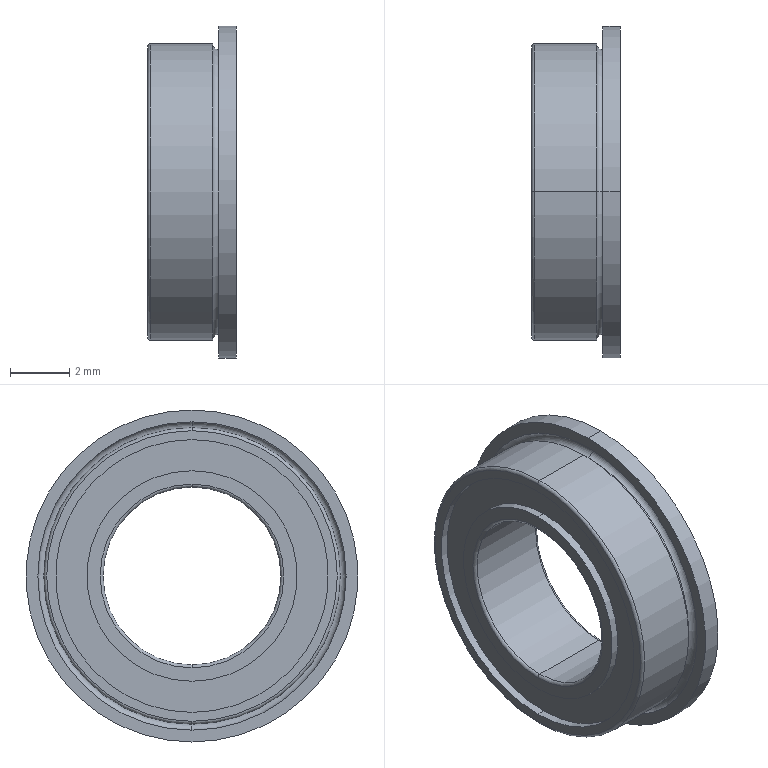Part | NX | features BREP 1 | 1 solid | 31 faces | box 3 x 11.2 x 11.2 mm | volume 145.175 mm3 | cylinder 14 | torus 10 | plane 7 | commonest cylinder face diameters 7.1 x4 9.2 x4 6 x2 10 x2 11.2 x2
STEP:
#1=CARTESIAN_POINT('',(0.,0.,4.8));
#2=VERTEX_POINT('',#1);
#3=CARTESIAN_POINT('',(-0.2,0.,5.));
#4=VERTEX_POINT('',#3);
#5=CARTESIAN_POINT('',(0.,0.,5.));
#6=DIRECTION('',(0.,-1.,0.));
#7=DIRECTION('',(0.,0.,-1.));
#8=AXIS2_PLACEMENT_3D('',#5,#6,#7);
#9=CIRCLE('',#8,0.2);
#10=EDGE_CURVE('',#2,#4,#9,.F.);
#11=ORIENTED_EDGE('',*,*,#10,.F.);
#12=CARTESIAN_POINT('',(0.,0.,-4.8));
#13=VERTEX_POINT('',#12);
#14=CARTESIAN_POINT('',(0.,0.,0.));
#15=DIRECTION('',(-1.,0.,0.));
#16=DIRECTION('',(0.,0.,1.));
#17=AXIS2_PLACEMENT_3D('',#14,#15,#16);
#18=CIRCLE('',#17,4.8);
#19=EDGE_CURVE('',#2,#13,#18,.T.);
#20=ORIENTED_EDGE('',*,*,#19,.T.);
#21=CARTESIAN_POINT('',(-0.2,0.,-5.));
#22=VERTEX_POINT('',#21);
#23=CARTESIAN_POINT('',(0.,0.,-5.));
#24=DIRECTION('',(0.,1.,0.));
#25=DIRECTION('',(0.,0.,1.));
#26=AXIS2_PLACEMENT_3D('',#23,#24,#25);
#27=CIRCLE('',#26,0.2);
#28=EDGE_CURVE('',#13,#22,#27,.F.);
#29=ORIENTED_EDGE('',*,*,#28,.T.);
#30=CARTESIAN_POINT('',(-0.2,0.,0.));
#31=DIRECTION('',(-1.,0.,0.));
#32=DIRECTION('',(0.,0.,1.));
#33=AXIS2_PLACEMENT_3D('',#30,#31,#32);
#34=CIRCLE('',#33,5.);
#35=EDGE_CURVE('',#4,#22,#34,.T.);
#36=ORIENTED_EDGE('',*,*,#35,.F.);
#37=EDGE_LOOP('',(#11,#20,#29,#36));
#38=FACE_BOUND('',#37,.T.);
#39=CARTESIAN_POINT('',(0.,0.,0.));
#40=DIRECTION('',(-1.,0.,0.));
#41=DIRECTION('',(0.,0.,-1.));
#42=AXIS2_PLACEMENT_3D('',#39,#40,#41);
#43=TOROIDAL_SURFACE('',#42,5.,0.2);
#44=ADVANCED_FACE('',(#38),#43,.F.);
#45=ORIENTED_EDGE('',*,*,#28,.F.);
#46=CARTESIAN_POINT('',(0.,0.,0.));
#47=DIRECTION('',(-1.,0.,0.));
#48=DIRECTION('',(0.,0.,1.));
#49=AXIS2_PLACEMENT_3D('',#46,#47,#48);
#50=CIRCLE('',#49,4.8);
#51=EDGE_CURVE('',#13,#2,#50,.T.);
#52=ORIENTED_EDGE('',*,*,#51,.T.);
#53=ORIENTED_EDGE('',*,*,#10,.T.);
#54=CARTESIAN_POINT('',(-0.2,0.,0.));
#55=DIRECTION('',(-1.,0.,0.));
#56=DIRECTION('',(0.,0.,1.));
#57=AXIS2_PLACEMENT_3D('',#54,#55,#56);
#58=CIRCLE('',#57,5.);
#59=EDGE_CURVE('',#22,#4,#58,.T.);
#60=ORIENTED_EDGE('',*,*,#59,.F.);
#61=EDGE_LOOP('',(#45,#52,#53,#60));
#62=FACE_BOUND('',#61,.T.);
#63=CARTESIAN_POINT('',(0.,0.,0.));
#64=DIRECTION('',(-1.,0.,0.));
#65=DIRECTION('',(0.,0.,-1.));
#66=AXIS2_PLACEMENT_3D('',#63,#64,#65);
#67=TOROIDAL_SURFACE('',#66,5.,0.2);
#68=ADVANCED_FACE('',(#62),#67,.F.);
#69=CARTESIAN_POINT('',(0.6,0.,-4.6));
#70=VERTEX_POINT('',#69);
#71=CARTESIAN_POINT('',(0.6,0.,4.6));
#72=VERTEX_POINT('',#71);
#73=CARTESIAN_POINT('',(0.6,0.,0.));
#74=DIRECTION('',(-1.,0.,0.));
#75=DIRECTION('',(0.,0.,1.));
#76=AXIS2_PLACEMENT_3D('',#73,#74,#75);
#77=CIRCLE('',#76,4.6);
#78=EDGE_CURVE('',#70,#72,#77,.T.);
#79=ORIENTED_EDGE('',*,*,#78,.F.);
#80=CARTESIAN_POINT('',(0.33,0.,-4.6));
#81=VERTEX_POINT('',#80);
#82=CARTESIAN_POINT('',(-1.815,0.,-4.6));
#83=DIRECTION('',(-1.,0.,0.));
#84=VECTOR('',#83,1000.);
#85=LINE('',#82,#84);
#86=EDGE_CURVE('',#70,#81,#85,.T.);
#87=ORIENTED_EDGE('',*,*,#86,.T.);
#88=CARTESIAN_POINT('',(0.33,0.,4.6));
#89=VERTEX_POINT('',#88);
#90=CARTESIAN_POINT('',(0.33,0.,0.));
#91=DIRECTION('',(-1.,0.,0.));
#92=DIRECTION('',(0.,0.,1.));
#93=AXIS2_PLACEMENT_3D('',#90,#91,#92);
#94=CIRCLE('',#93,4.6);
#95=EDGE_CURVE('',#81,#89,#94,.T.);
#96=ORIENTED_EDGE('',*,*,#95,.T.);
#97=CARTESIAN_POINT('',(-1.815,0.,4.6));
#98=DIRECTION('',(-1.,0.,0.));
#99=VECTOR('',#98,1000.);
#100=LINE('',#97,#99);
#101=EDGE_CURVE('',#72,#89,#100,.T.);
#102=ORIENTED_EDGE('',*,*,#101,.F.);
#103=EDGE_LOOP('',(#79,#87,#96,#102));
#104=FACE_BOUND('',#103,.T.);
#105=CARTESIAN_POINT('',(-1.815,0.,0.));
#106=DIRECTION('',(-1.,0.,0.));
#107=DIRECTION('',(0.,0.,-1.));
#108=AXIS2_PLACEMENT_3D('',#105,#106,#107);
#109=CYLINDRICAL_SURFACE('',#108,4.6);
#110=ADVANCED_FACE('',(#104),#109,.F.);
#111=CARTESIAN_POINT('',(0.6,0.,3.55));
#112=VERTEX_POINT('',#111);
#113=CARTESIAN_POINT('',(0.6,0.,-3.55));
#114=VERTEX_POINT('',#113);
#115=CARTESIAN_POINT('',(0.6,0.,0.));
#116=DIRECTION('',(-1.,0.,0.));
#117=DIRECTION('',(0.,0.,1.));
#118=AXIS2_PLACEMENT_3D('',#115,#116,#117);
#119=CIRCLE('',#118,3.55);
#120=EDGE_CURVE('',#112,#114,#119,.T.);
#121=ORIENTED_EDGE('',*,*,#120,.T.);
#122=CARTESIAN_POINT('',(0.33,0.,-3.55));
#123=VERTEX_POINT('',#122);
#124=CARTESIAN_POINT('',(-1.815,0.,-3.55));
#125=DIRECTION('',(-1.,0.,0.));
#126=VECTOR('',#125,1000.);
#127=LINE('',#124,#126);
#128=EDGE_CURVE('',#114,#123,#127,.T.);
#129=ORIENTED_EDGE('',*,*,#128,.T.);
#130=CARTESIAN_POINT('',(0.33,0.,3.55));
#131=VERTEX_POINT('',#130);
#132=CARTESIAN_POINT('',(0.33,0.,0.));
#133=DIRECTION('',(-1.,0.,0.));
#134=DIRECTION('',(0.,0.,1.));
#135=AXIS2_PLACEMENT_3D('',#132,#133,#134);
#136=CIRCLE('',#135,3.55);
#137=EDGE_CURVE('',#131,#123,#136,.T.);
#138=ORIENTED_EDGE('',*,*,#137,.F.);
#139=CARTESIAN_POINT('',(-1.815,0.,3.55));
#140=DIRECTION('',(-1.,0.,0.));
#141=VECTOR('',#140,1000.);
#142=LINE('',#139,#141);
#143=EDGE_CURVE('',#112,#131,#142,.T.);
#144=ORIENTED_EDGE('',*,*,#143,.F.);
#145=EDGE_LOOP('',(#121,#129,#138,#144));
#146=FACE_BOUND('',#145,.T.);
#147=CARTESIAN_POINT('',(-1.815,0.,0.));
#148=DIRECTION('',(-1.,0.,0.));
#149=DIRECTION('',(0.,0.,-1.));
#150=AXIS2_PLACEMENT_3D('',#147,#148,#149);
#151=CYLINDRICAL_SURFACE('',#150,3.55);
#152=ADVANCED_FACE('',(#146),#151,.T.);
#153=CARTESIAN_POINT('',(0.5,0.,3.));
#154=VERTEX_POINT('',#153);
#155=CARTESIAN_POINT('',(0.5,0.,-3.));
#156=VERTEX_POINT('',#155);
#157=CARTESIAN_POINT('',(0.5,0.,0.));
#158=DIRECTION('',(-1.,0.,0.));
#159=DIRECTION('',(0.,0.,1.));
#160=AXIS2_PLACEMENT_3D('',#157,#158,#159);
#161=CIRCLE('',#160,3.);
#162=EDGE_CURVE('',#154,#156,#161,.T.);
#163=ORIENTED_EDGE('',*,*,#162,.T.);
#164=CARTESIAN_POINT('',(0.6,0.,-3.1));
#165=VERTEX_POINT('',#164);
#166=CARTESIAN_POINT('',(0.5,0.,-3.1));
#167=DIRECTION('',(0.,1.,0.));
#168=DIRECTION('',(0.,0.,1.));
#169=AXIS2_PLACEMENT_3D('',#166,#167,#168);
#170=CIRCLE('',#169,0.1);
#171=EDGE_CURVE('',#156,#165,#170,.T.);
#172=ORIENTED_EDGE('',*,*,#171,.T.);
#173=CARTESIAN_POINT('',(0.6,0.,3.1));
#174=VERTEX_POINT('',#173);
#175=CARTESIAN_POINT('',(0.6,0.,0.));
#176=DIRECTION('',(-1.,0.,0.));
#177=DIRECTION('',(0.,0.,1.));
#178=AXIS2_PLACEMENT_3D('',#175,#176,#177);
#179=CIRCLE('',#178,3.1);
#180=EDGE_CURVE('',#174,#165,#179,.T.);
#181=ORIENTED_EDGE('',*,*,#180,.F.);
#182=CARTESIAN_POINT('',(0.5,0.,3.1));
#183=DIRECTION('',(0.,-1.,0.));
#184=DIRECTION('',(0.,0.,-1.));
#185=AXIS2_PLACEMENT_3D('',#182,#183,#184);
#186=CIRCLE('',#185,0.1);
#187=EDGE_CURVE('',#154,#174,#186,.T.);
#188=ORIENTED_EDGE('',*,*,#187,.F.);
#189=EDGE_LOOP('',(#163,#172,#181,#188));
#190=FACE_BOUND('',#189,.T.);
#191=CARTESIAN_POINT('',(0.5,0.,0.));
#192=DIRECTION('',(-1.,0.,0.));
#193=DIRECTION('',(0.,0.,-1.));
#194=AXIS2_PLACEMENT_3D('',#191,#192,#193);
#195=TOROIDAL_SURFACE('',#194,3.1,0.1);
#196=ADVANCED_FACE('',(#190),#195,.T.);
#197=CARTESIAN_POINT('',(0.5,0.,0.));
#198=DIRECTION('',(-1.,0.,0.));
#199=DIRECTION('',(0.,0.,1.));
#200=AXIS2_PLACEMENT_3D('',#197,#198,#199);
#201=CIRCLE('',#200,3.);
#202=EDGE_CURVE('',#156,#154,#201,.T.);
#203=ORIENTED_EDGE('',*,*,#202,.F.);
#204=CARTESIAN_POINT('',(-2.3,0.,-3.));
#205=VERTEX_POINT('',#204);
#206=CARTESIAN_POINT('',(-1.815,0.,-3.));
#207=DIRECTION('',(-1.,0.,0.));
#208=VECTOR('',#207,1000.);
#209=LINE('',#206,#208);
#210=EDGE_CURVE('',#156,#205,#209,.T.);
#211=ORIENTED_EDGE('',*,*,#210,.T.);
#212=CARTESIAN_POINT('',(-2.3,0.,3.));
#213=VERTEX_POINT('',#212);
#214=CARTESIAN_POINT('',(-2.3,0.,0.));
#215=DIRECTION('',(-1.,0.,0.));
#216=DIRECTION('',(0.,0.,1.));
#217=AXIS2_PLACEMENT_3D('',#214,#215,#216);
#218=CIRCLE('',#217,3.);
#219=EDGE_CURVE('',#205,#213,#218,.T.);
#220=ORIENTED_EDGE('',*,*,#219,.T.);
#221=CARTESIAN_POINT('',(-1.815,0.,3.));
#222=DIRECTION('',(-1.,0.,0.));
#223=VECTOR('',#222,1000.);
#224=LINE('',#221,#223);
#225=EDGE_CURVE('',#154,#213,#224,.T.);
#226=ORIENTED_EDGE('',*,*,#225,.F.);
#227=EDGE_LOOP('',(#203,#211,#220,#226));
#228=FACE_BOUND('',#227,.T.);
#229=CARTESIAN_POINT('',(-1.815,0.,0.));
#230=DIRECTION('',(-1.,0.,0.));
#231=DIRECTION('',(0.,0.,-1.));
#232=AXIS2_PLACEMENT_3D('',#229,#230,#231);
#233=CYLINDRICAL_SURFACE('',#232,3.);
#234=ADVANCED_FACE('',(#228),#233,.F.);
#235=CARTESIAN_POINT('',(-2.4,0.,3.1));
#236=VERTEX_POINT('',#235);
#237=CARTESIAN_POINT('',(-2.4,0.,-3.1));
#238=VERTEX_POINT('',#237);
#239=CARTESIAN_POINT('',(-2.4,0.,0.));
#240=DIRECTION('',(-1.,0.,0.));
#241=DIRECTION('',(0.,0.,1.));
#242=AXIS2_PLACEMENT_3D('',#239,#240,#241);
#243=CIRCLE('',#242,3.1);
#244=EDGE_CURVE('',#236,#238,#243,.T.);
#245=ORIENTED_EDGE('',*,*,#244,.T.);
#246=CARTESIAN_POINT('',(-2.3,0.,-3.1));
#247=DIRECTION('',(0.,1.,0.));
#248=DIRECTION('',(0.,0.,1.));
#249=AXIS2_PLACEMENT_3D('',#246,#247,#248);
#250=CIRCLE('',#249,0.1);
#251=EDGE_CURVE('',#238,#205,#250,.T.);
#252=ORIENTED_EDGE('',*,*,#251,.T.);
#253=CARTESIAN_POINT('',(-2.3,0.,0.));
#254=DIRECTION('',(-1.,0.,0.));
#255=DIRECTION('',(0.,0.,1.));
#256=AXIS2_PLACEMENT_3D('',#253,#254,#255);
#257=CIRCLE('',#256,3.);
#258=EDGE_CURVE('',#213,#205,#257,.T.);
#259=ORIENTED_EDGE('',*,*,#258,.F.);
#260=CARTESIAN_POINT('',(-2.3,0.,3.1));
#261=DIRECTION('',(0.,-1.,0.));
#262=DIRECTION('',(0.,0.,-1.));
#263=AXIS2_PLACEMENT_3D('',#260,#261,#262);
#264=CIRCLE('',#263,0.1);
#265=EDGE_CURVE('',#236,#213,#264,.T.);
#266=ORIENTED_EDGE('',*,*,#265,.F.);
#267=EDGE_LOOP('',(#245,#252,#259,#266));
#268=FACE_BOUND('',#267,.T.);
#269=CARTESIAN_POINT('',(-2.3,0.,0.));
#270=DIRECTION('',(-1.,0.,0.));
#271=DIRECTION('',(0.,0.,-1.));
#272=AXIS2_PLACEMENT_3D('',#269,#270,#271);
#273=TOROIDAL_SURFACE('',#272,3.1,0.1);
#274=ADVANCED_FACE('',(#268),#273,.T.);
#275=CARTESIAN_POINT('',(-2.13,0.,3.55));
#276=VERTEX_POINT('',#275);
#277=CARTESIAN_POINT('',(-2.13,0.,-3.55));
#278=VERTEX_POINT('',#277);
#279=CARTESIAN_POINT('',(-2.13,0.,0.));
#280=DIRECTION('',(-1.,0.,0.));
#281=DIRECTION('',(0.,0.,1.));
#282=AXIS2_PLACEMENT_3D('',#279,#280,#281);
#283=CIRCLE('',#282,3.55);
#284=EDGE_CURVE('',#276,#278,#283,.T.);
#285=ORIENTED_EDGE('',*,*,#284,.T.);
#286=CARTESIAN_POINT('',(-2.4,0.,-3.55));
#287=VERTEX_POINT('',#286);
#288=CARTESIAN_POINT('',(-1.815,0.,-3.55));
#289=DIRECTION('',(-1.,0.,0.));
#290=VECTOR('',#289,1000.);
#291=LINE('',#288,#290);
#292=EDGE_CURVE('',#278,#287,#291,.T.);
#293=ORIENTED_EDGE('',*,*,#292,.T.);
#294=CARTESIAN_POINT('',(-2.4,0.,3.55));
#295=VERTEX_POINT('',#294);
#296=CARTESIAN_POINT('',(-2.4,0.,0.));
#297=DIRECTION('',(-1.,0.,0.));
#298=DIRECTION('',(0.,0.,1.));
#299=AXIS2_PLACEMENT_3D('',#296,#297,#298);
#300=CIRCLE('',#299,3.55);
#301=EDGE_CURVE('',#295,#287,#300,.T.);
#302=ORIENTED_EDGE('',*,*,#301,.F.);
#303=CARTESIAN_POINT('',(-1.815,0.,3.55));
#304=DIRECTION('',(-1.,0.,0.));
#305=VECTOR('',#304,1000.);
#306=LINE('',#303,#305);
#307=EDGE_CURVE('',#276,#295,#306,.T.);
#308=ORIENTED_EDGE('',*,*,#307,.F.);
#309=EDGE_LOOP('',(#285,#293,#302,#308));
#310=FACE_BOUND('',#309,.T.);
#311=CARTESIAN_POINT('',(-1.815,0.,0.));
#312=DIRECTION('',(-1.,0.,0.));
#313=DIRECTION('',(0.,0.,-1.));
#314=AXIS2_PLACEMENT_3D('',#311,#312,#313);
#315=CYLINDRICAL_SURFACE('',#314,3.55);
#316=ADVANCED_FACE('',(#310),#315,.T.);
#317=CARTESIAN_POINT('',(-2.13,0.,-4.6));
#318=VERTEX_POINT('',#317);
#319=CARTESIAN_POINT('',(-2.13,0.,4.6));
#320=VERTEX_POINT('',#319);
#321=CARTESIAN_POINT('',(-2.13,0.,0.));
#322=DIRECTION('',(-1.,0.,0.));
#323=DIRECTION('',(0.,0.,1.));
#324=AXIS2_PLACEMENT_3D('',#321,#322,#323);
#325=CIRCLE('',#324,4.6);
#326=EDGE_CURVE('',#318,#320,#325,.T.);
#327=ORIENTED_EDGE('',*,*,#326,.F.);
#328=CARTESIAN_POINT('',(-2.4,0.,-4.6));
#329=VERTEX_POINT('',#328);
#330=CARTESIAN_POINT('',(-1.815,0.,-4.6));
#331=DIRECTION('',(-1.,0.,0.));
#332=VECTOR('',#331,1000.);
#333=LINE('',#330,#332);
#334=EDGE_CURVE('',#318,#329,#333,.T.);
#335=ORIENTED_EDGE('',*,*,#334,.T.);
#336=CARTESIAN_POINT('',(-2.4,0.,4.6));
#337=VERTEX_POINT('',#336);
#338=CARTESIAN_POINT('',(-2.4,0.,0.));
#339=DIRECTION('',(-1.,0.,0.));
#340=DIRECTION('',(0.,0.,1.));
#341=AXIS2_PLACEMENT_3D('',#338,#339,#340);
#342=CIRCLE('',#341,4.6);
#343=EDGE_CURVE('',#329,#337,#342,.T.);
#344=ORIENTED_EDGE('',*,*,#343,.T.);
#345=CARTESIAN_POINT('',(-1.815,0.,4.6));
#346=DIRECTION('',(-1.,0.,0.));
#347=VECTOR('',#346,1000.);
#348=LINE('',#345,#347);
#349=EDGE_CURVE('',#320,#337,#348,.T.);
#350=ORIENTED_EDGE('',*,*,#349,.F.);
#351=EDGE_LOOP('',(#327,#335,#344,#350));
#352=FACE_BOUND('',#351,.T.);
#353=CARTESIAN_POINT('',(-1.815,0.,0.));
#354=DIRECTION('',(-1.,0.,0.));
#355=DIRECTION('',(0.,0.,-1.));
#356=AXIS2_PLACEMENT_3D('',#353,#354,#355);
#357=CYLINDRICAL_SURFACE('',#356,4.6);
#358=ADVANCED_FACE('',(#352),#357,.F.);
#359=CARTESIAN_POINT('',(-2.3,0.,5.));
#360=VERTEX_POINT('',#359);
#361=CARTESIAN_POINT('',(-2.3,0.,-5.));
#362=VERTEX_POINT('',#361);
#363=CARTESIAN_POINT('',(-2.3,0.,0.));
#364=DIRECTION('',(-1.,0.,0.));
#365=DIRECTION('',(0.,0.,1.));
#366=AXIS2_PLACEMENT_3D('',#363,#364,#365);
#367=CIRCLE('',#366,5.);
#368=EDGE_CURVE('',#360,#362,#367,.T.);
#369=ORIENTED_EDGE('',*,*,#368,.T.);
#370=CARTESIAN_POINT('',(-2.4,0.,-4.9));
#371=VERTEX_POINT('',#370);
#372=CARTESIAN_POINT('',(-2.3,0.,-4.9));
#373=DIRECTION('',(0.,1.,0.));
#374=DIRECTION('',(0.,0.,1.));
#375=AXIS2_PLACEMENT_3D('',#372,#373,#374);
#376=CIRCLE('',#375,0.1);
#377=EDGE_CURVE('',#362,#371,#376,.T.);
#378=ORIENTED_EDGE('',*,*,#377,.T.);
#379=CARTESIAN_POINT('',(-2.4,0.,4.9));
#380=VERTEX_POINT('',#379);
#381=CARTESIAN_POINT('',(-2.4,0.,0.));
#382=DIRECTION('',(-1.,0.,0.));
#383=DIRECTION('',(0.,0.,1.));
#384=AXIS2_PLACEMENT_3D('',#381,#382,#383);
#385=CIRCLE('',#384,4.9);
#386=EDGE_CURVE('',#380,#371,#385,.T.);
#387=ORIENTED_EDGE('',*,*,#386,.F.);
#388=CARTESIAN_POINT('',(-2.3,0.,4.9));
#389=DIRECTION('',(0.,-1.,0.));
#390=DIRECTION('',(0.,0.,-1.));
#391=AXIS2_PLACEMENT_3D('',#388,#389,#390);
#392=CIRCLE('',#391,0.1);
#393=EDGE_CURVE('',#360,#380,#392,.T.);
#394=ORIENTED_EDGE('',*,*,#393,.F.);
#395=EDGE_LOOP('',(#369,#378,#387,#394));
#396=FACE_BOUND('',#395,.T.);
#397=CARTESIAN_POINT('',(-2.3,0.,0.));
#398=DIRECTION('',(-1.,0.,0.));
#399=DIRECTION('',(0.,0.,-1.));
#400=AXIS2_PLACEMENT_3D('',#397,#398,#399);
#401=TOROIDAL_SURFACE('',#400,4.9,0.1);
#402=ADVANCED_FACE('',(#396),#401,.T.);
#403=ORIENTED_EDGE('',*,*,#35,.T.);
#404=CARTESIAN_POINT('',(-1.815,0.,-5.));
#405=DIRECTION('',(-1.,0.,0.));
#406=VECTOR('',#405,1000.);
#407=LINE('',#404,#406);
#408=EDGE_CURVE('',#22,#362,#407,.T.);
#409=ORIENTED_EDGE('',*,*,#408,.T.);
#410=ORIENTED_EDGE('',*,*,#368,.F.);
#411=CARTESIAN_POINT('',(-1.815,0.,5.));
#412=DIRECTION('',(-1.,0.,0.));
#413=VECTOR('',#412,1000.);
#414=LINE('',#411,#413);
#415=EDGE_CURVE('',#4,#360,#414,.T.);
#416=ORIENTED_EDGE('',*,*,#415,.F.);
#417=EDGE_LOOP('',(#403,#409,#410,#416));
#418=FACE_BOUND('',#417,.T.);
#419=CARTESIAN_POINT('',(-1.815,0.,0.));
#420=DIRECTION('',(-1.,0.,0.));
#421=DIRECTION('',(0.,0.,-1.));
#422=AXIS2_PLACEMENT_3D('',#419,#420,#421);
#423=CYLINDRICAL_SURFACE('',#422,5.);
#424=ADVANCED_FACE('',(#418),#423,.T.);
#425=ORIENTED_EDGE('',*,*,#51,.F.);
#426=CARTESIAN_POINT('',(0.,0.,-5.2));
#427=VERTEX_POINT('',#426);
#428=CARTESIAN_POINT('',(0.,0.,-5.));
#429=DIRECTION('',(0.,1.,0.));
#430=DIRECTION('',(0.,0.,1.));
#431=AXIS2_PLACEMENT_3D('',#428,#429,#430);
#432=CIRCLE('',#431,0.2);
#433=EDGE_CURVE('',#13,#427,#432,.T.);
#434=ORIENTED_EDGE('',*,*,#433,.T.);
#435=CARTESIAN_POINT('',(0.,0.,5.2));
#436=VERTEX_POINT('',#435);
#437=CARTESIAN_POINT('',(0.,0.,0.));
#438=DIRECTION('',(-1.,0.,0.));
#439=DIRECTION('',(0.,0.,1.));
#440=AXIS2_PLACEMENT_3D('',#437,#438,#439);
#441=CIRCLE('',#440,5.2);
#442=EDGE_CURVE('',#427,#436,#441,.T.);
#443=ORIENTED_EDGE('',*,*,#442,.T.);
#444=CARTESIAN_POINT('',(0.,0.,5.));
#445=DIRECTION('',(0.,-1.,0.));
#446=DIRECTION('',(0.,0.,-1.));
#447=AXIS2_PLACEMENT_3D('',#444,#445,#446);
#448=CIRCLE('',#447,0.2);
#449=EDGE_CURVE('',#2,#436,#448,.T.);
#450=ORIENTED_EDGE('',*,*,#449,.F.);
#451=EDGE_LOOP('',(#425,#434,#443,#450));
#452=FACE_BOUND('',#451,.T.);
#453=CARTESIAN_POINT('',(0.,0.,0.));
#454=DIRECTION('',(-1.,0.,0.));
#455=DIRECTION('',(0.,0.,-1.));
#456=AXIS2_PLACEMENT_3D('',#453,#454,#455);
#457=TOROIDAL_SURFACE('',#456,5.,0.2);
#458=ADVANCED_FACE('',(#452),#457,.F.);
#459=CARTESIAN_POINT('',(0.6,0.,5.6));
#460=VERTEX_POINT('',#459);
#461=CARTESIAN_POINT('',(0.6,0.,-5.6));
#462=VERTEX_POINT('',#461);
#463=CARTESIAN_POINT('',(0.6,0.,0.));
#464=DIRECTION('',(-1.,0.,0.));
#465=DIRECTION('',(0.,0.,1.));
#466=AXIS2_PLACEMENT_3D('',#463,#464,#465);
#467=CIRCLE('',#466,5.6);
#468=EDGE_CURVE('',#460,#462,#467,.T.);
#469=ORIENTED_EDGE('',*,*,#468,.T.);
#470=CARTESIAN_POINT('',(0.,0.,-5.6));
#471=VERTEX_POINT('',#470);
#472=CARTESIAN_POINT('',(-1.815,0.,-5.6));
#473=DIRECTION('',(-1.,0.,0.));
#474=VECTOR('',#473,1000.);
#475=LINE('',#472,#474);
#476=EDGE_CURVE('',#462,#471,#475,.T.);
#477=ORIENTED_EDGE('',*,*,#476,.T.);
#478=CARTESIAN_POINT('',(0.,0.,5.6));
#479=VERTEX_POINT('',#478);
#480=CARTESIAN_POINT('',(0.,0.,0.));
#481=DIRECTION('',(-1.,0.,0.));
#482=DIRECTION('',(0.,0.,1.));
#483=AXIS2_PLACEMENT_3D('',#480,#481,#482);
#484=CIRCLE('',#483,5.6);
#485=EDGE_CURVE('',#479,#471,#484,.T.);
#486=ORIENTED_EDGE('',*,*,#485,.F.);
#487=CARTESIAN_POINT('',(-1.815,0.,5.6));
#488=DIRECTION('',(-1.,0.,0.));
#489=VECTOR('',#488,1000.);
#490=LINE('',#487,#489);
#491=EDGE_CURVE('',#460,#479,#490,.T.);
#492=ORIENTED_EDGE('',*,*,#491,.F.);
#493=EDGE_LOOP('',(#469,#477,#486,#492));
#494=FACE_BOUND('',#493,.T.);
#495=CARTESIAN_POINT('',(-1.815,0.,0.));
#496=DIRECTION('',(-1.,0.,0.));
#497=DIRECTION('',(0.,0.,-1.));
#498=AXIS2_PLACEMENT_3D('',#495,#496,#497);
#499=CYLINDRICAL_SURFACE('',#498,5.6);
#500=ADVANCED_FACE('',(#494),#499,.T.);
#501=ORIENTED_EDGE('',*,*,#476,.F.);
#502=CARTESIAN_POINT('',(0.6,0.,0.));
#503=DIRECTION('',(-1.,0.,0.));
#504=DIRECTION('',(0.,0.,1.));
#505=AXIS2_PLACEMENT_3D('',#502,#503,#504);
#506=CIRCLE('',#505,5.6);
#507=EDGE_CURVE('',#462,#460,#506,.T.);
#508=ORIENTED_EDGE('',*,*,#507,.T.);
#509=ORIENTED_EDGE('',*,*,#491,.T.);
#510=CARTESIAN_POINT('',(0.,0.,0.));
#511=DIRECTION('',(-1.,0.,0.));
#512=DIRECTION('',(0.,0.,1.));
#513=AXIS2_PLACEMENT_3D('',#510,#511,#512);
#514=CIRCLE('',#513,5.6);
#515=EDGE_CURVE('',#471,#479,#514,.T.);
#516=ORIENTED_EDGE('',*,*,#515,.F.);
#517=EDGE_LOOP('',(#501,#508,#509,#516));
#518=FACE_BOUND('',#517,.T.);
#519=CARTESIAN_POINT('',(-1.815,0.,0.));
#520=DIRECTION('',(-1.,0.,0.));
#521=DIRECTION('',(0.,0.,-1.));
#522=AXIS2_PLACEMENT_3D('',#519,#520,#521);
#523=CYLINDRICAL_SURFACE('',#522,5.6);
#524=ADVANCED_FACE('',(#518),#523,.T.);
#525=ORIENTED_EDGE('',*,*,#485,.T.);
#526=ORIENTED_EDGE('',*,*,#515,.T.);
#527=EDGE_LOOP('',(#525,#526));
#528=FACE_BOUND('',#527,.T.);
#529=CARTESIAN_POINT('',(0.,0.,0.));
#530=DIRECTION('',(-1.,0.,0.));
#531=DIRECTION('',(0.,0.,1.));
#532=AXIS2_PLACEMENT_3D('',#529,#530,#531);
#533=CIRCLE('',#532,5.2);
#534=EDGE_CURVE('',#436,#427,#533,.T.);
#535=ORIENTED_EDGE('',*,*,#534,.F.);
#536=ORIENTED_EDGE('',*,*,#442,.F.);
#537=EDGE_LOOP('',(#535,#536));
#538=FACE_BOUND('',#537,.T.);
#539=CARTESIAN_POINT('',(0.,5.2,0.));
#540=DIRECTION('',(1.,0.,0.));
#541=DIRECTION('',(0.,-1.,0.));
#542=AXIS2_PLACEMENT_3D('',#539,#540,#541);
#543=PLANE('',#542);
#544=ADVANCED_FACE('',(#528,#538),#543,.F.);
#545=ORIENTED_EDGE('',*,*,#19,.F.);
#546=ORIENTED_EDGE('',*,*,#449,.T.);
#547=ORIENTED_EDGE('',*,*,#534,.T.);
#548=ORIENTED_EDGE('',*,*,#433,.F.);
#549=EDGE_LOOP('',(#545,#546,#547,#548));
#550=FACE_BOUND('',#549,.T.);
#551=CARTESIAN_POINT('',(0.,0.,0.));
#552=DIRECTION('',(-1.,0.,0.));
#553=DIRECTION('',(0.,0.,-1.));
#554=AXIS2_PLACEMENT_3D('',#551,#552,#553);
#555=TOROIDAL_SURFACE('',#554,5.,0.2);
#556=ADVANCED_FACE('',(#550),#555,.F.);
#557=ORIENTED_EDGE('',*,*,#408,.F.);
#558=ORIENTED_EDGE('',*,*,#59,.T.);
#559=ORIENTED_EDGE('',*,*,#415,.T.);
#560=CARTESIAN_POINT('',(-2.3,0.,0.));
#561=DIRECTION('',(-1.,0.,0.));
#562=DIRECTION('',(0.,0.,1.));
#563=AXIS2_PLACEMENT_3D('',#560,#561,#562);
#564=CIRCLE('',#563,5.);
#565=EDGE_CURVE('',#362,#360,#564,.T.);
#566=ORIENTED_EDGE('',*,*,#565,.F.);
#567=EDGE_LOOP('',(#557,#558,#559,#566));
#568=FACE_BOUND('',#567,.T.);
#569=CARTESIAN_POINT('',(-1.815,0.,0.));
#570=DIRECTION('',(-1.,0.,0.));
#571=DIRECTION('',(0.,0.,-1.));
#572=AXIS2_PLACEMENT_3D('',#569,#570,#571);
#573=CYLINDRICAL_SURFACE('',#572,5.);
#574=ADVANCED_FACE('',(#568),#573,.T.);
#575=ORIENTED_EDGE('',*,*,#377,.F.);
#576=ORIENTED_EDGE('',*,*,#565,.T.);
#577=ORIENTED_EDGE('',*,*,#393,.T.);
#578=CARTESIAN_POINT('',(-2.4,0.,0.));
#579=DIRECTION('',(-1.,0.,0.));
#580=DIRECTION('',(0.,0.,1.));
#581=AXIS2_PLACEMENT_3D('',#578,#579,#580);
#582=CIRCLE('',#581,4.9);
#583=EDGE_CURVE('',#371,#380,#582,.T.);
#584=ORIENTED_EDGE('',*,*,#583,.F.);
#585=EDGE_LOOP('',(#575,#576,#577,#584));
#586=FACE_BOUND('',#585,.T.);
#587=CARTESIAN_POINT('',(-2.3,0.,0.));
#588=DIRECTION('',(-1.,0.,0.));
#589=DIRECTION('',(0.,0.,-1.));
#590=AXIS2_PLACEMENT_3D('',#587,#588,#589);
#591=TOROIDAL_SURFACE('',#590,4.9,0.1);
#592=ADVANCED_FACE('',(#586),#591,.T.);
#593=ORIENTED_EDGE('',*,*,#386,.T.);
#594=ORIENTED_EDGE('',*,*,#583,.T.);
#595=EDGE_LOOP('',(#593,#594));
#596=FACE_BOUND('',#595,.T.);
#597=CARTESIAN_POINT('',(-2.4,0.,0.));
#598=DIRECTION('',(-1.,0.,0.));
#599=DIRECTION('',(0.,0.,1.));
#600=AXIS2_PLACEMENT_3D('',#597,#598,#599);
#601=CIRCLE('',#600,4.6);
#602=EDGE_CURVE('',#337,#329,#601,.T.);
#603=ORIENTED_EDGE('',*,*,#602,.F.);
#604=ORIENTED_EDGE('',*,*,#343,.F.);
#605=EDGE_LOOP('',(#603,#604));
#606=FACE_BOUND('',#605,.T.);
#607=CARTESIAN_POINT('',(-2.4,4.6,0.));
#608=DIRECTION('',(1.,0.,0.));
#609=DIRECTION('',(0.,-1.,0.));
#610=AXIS2_PLACEMENT_3D('',#607,#608,#609);
#611=PLANE('',#610);
#612=ADVANCED_FACE('',(#596,#606),#611,.F.);
#613=ORIENTED_EDGE('',*,*,#334,.F.);
#614=CARTESIAN_POINT('',(-2.13,0.,0.));
#615=DIRECTION('',(-1.,0.,0.));
#616=DIRECTION('',(0.,0.,1.));
#617=AXIS2_PLACEMENT_3D('',#614,#615,#616);
#618=CIRCLE('',#617,4.6);
#619=EDGE_CURVE('',#320,#318,#618,.T.);
#620=ORIENTED_EDGE('',*,*,#619,.F.);
#621=ORIENTED_EDGE('',*,*,#349,.T.);
#622=ORIENTED_EDGE('',*,*,#602,.T.);
#623=EDGE_LOOP('',(#613,#620,#621,#622));
#624=FACE_BOUND('',#623,.T.);
#625=CARTESIAN_POINT('',(-1.815,0.,0.));
#626=DIRECTION('',(-1.,0.,0.));
#627=DIRECTION('',(0.,0.,-1.));
#628=AXIS2_PLACEMENT_3D('',#625,#626,#627);
#629=CYLINDRICAL_SURFACE('',#628,4.6);
#630=ADVANCED_FACE('',(#624),#629,.F.);
#631=ORIENTED_EDGE('',*,*,#619,.T.);
#632=ORIENTED_EDGE('',*,*,#326,.T.);
#633=EDGE_LOOP('',(#631,#632));
#634=FACE_BOUND('',#633,.T.);
#635=ORIENTED_EDGE('',*,*,#284,.F.);
#636=CARTESIAN_POINT('',(-2.13,0.,0.));
#637=DIRECTION('',(-1.,0.,0.));
#638=DIRECTION('',(0.,0.,1.));
#639=AXIS2_PLACEMENT_3D('',#636,#637,#638);
#640=CIRCLE('',#639,3.55);
#641=EDGE_CURVE('',#278,#276,#640,.T.);
#642=ORIENTED_EDGE('',*,*,#641,.F.);
#643=EDGE_LOOP('',(#635,#642));
#644=FACE_BOUND('',#643,.T.);
#645=CARTESIAN_POINT('',(-2.13,4.6,0.));
#646=DIRECTION('',(1.,0.,0.));
#647=DIRECTION('',(0.,-1.,0.));
#648=AXIS2_PLACEMENT_3D('',#645,#646,#647);
#649=PLANE('',#648);
#650=ADVANCED_FACE('',(#634,#644),#649,.F.);
#651=ORIENTED_EDGE('',*,*,#292,.F.);
#652=ORIENTED_EDGE('',*,*,#641,.T.);
#653=ORIENTED_EDGE('',*,*,#307,.T.);
#654=CARTESIAN_POINT('',(-2.4,0.,0.));
#655=DIRECTION('',(-1.,0.,0.));
#656=DIRECTION('',(0.,0.,1.));
#657=AXIS2_PLACEMENT_3D('',#654,#655,#656);
#658=CIRCLE('',#657,3.55);
#659=EDGE_CURVE('',#287,#295,#658,.T.);
#660=ORIENTED_EDGE('',*,*,#659,.F.);
#661=EDGE_LOOP('',(#651,#652,#653,#660));
#662=FACE_BOUND('',#661,.T.);
#663=CARTESIAN_POINT('',(-1.815,0.,0.));
#664=DIRECTION('',(-1.,0.,0.));
#665=DIRECTION('',(0.,0.,-1.));
#666=AXIS2_PLACEMENT_3D('',#663,#664,#665);
#667=CYLINDRICAL_SURFACE('',#666,3.55);
#668=ADVANCED_FACE('',(#662),#667,.T.);
#669=ORIENTED_EDGE('',*,*,#301,.T.);
#670=ORIENTED_EDGE('',*,*,#659,.T.);
#671=EDGE_LOOP('',(#669,#670));
#672=FACE_BOUND('',#671,.T.);
#673=ORIENTED_EDGE('',*,*,#244,.F.);
#674=CARTESIAN_POINT('',(-2.4,0.,0.));
#675=DIRECTION('',(-1.,0.,0.));
#676=DIRECTION('',(0.,0.,1.));
#677=AXIS2_PLACEMENT_3D('',#674,#675,#676);
#678=CIRCLE('',#677,3.1);
#679=EDGE_CURVE('',#238,#236,#678,.T.);
#680=ORIENTED_EDGE('',*,*,#679,.F.);
#681=EDGE_LOOP('',(#673,#680));
#682=FACE_BOUND('',#681,.T.);
#683=CARTESIAN_POINT('',(-2.4,3.1,0.));
#684=DIRECTION('',(1.,0.,0.));
#685=DIRECTION('',(0.,-1.,0.));
#686=AXIS2_PLACEMENT_3D('',#683,#684,#685);
#687=PLANE('',#686);
#688=ADVANCED_FACE('',(#672,#682),#687,.F.);
#689=ORIENTED_EDGE('',*,*,#251,.F.);
#690=ORIENTED_EDGE('',*,*,#679,.T.);
#691=ORIENTED_EDGE('',*,*,#265,.T.);
#692=ORIENTED_EDGE('',*,*,#219,.F.);
#693=EDGE_LOOP('',(#689,#690,#691,#692));
#694=FACE_BOUND('',#693,.T.);
#695=CARTESIAN_POINT('',(-2.3,0.,0.));
#696=DIRECTION('',(-1.,0.,0.));
#697=DIRECTION('',(0.,0.,-1.));
#698=AXIS2_PLACEMENT_3D('',#695,#696,#697);
#699=TOROIDAL_SURFACE('',#698,3.1,0.1);
#700=ADVANCED_FACE('',(#694),#699,.T.);
#701=ORIENTED_EDGE('',*,*,#210,.F.);
#702=ORIENTED_EDGE('',*,*,#162,.F.);
#703=ORIENTED_EDGE('',*,*,#225,.T.);
#704=ORIENTED_EDGE('',*,*,#258,.T.);
#705=EDGE_LOOP('',(#701,#702,#703,#704));
#706=FACE_BOUND('',#705,.T.);
#707=CARTESIAN_POINT('',(-1.815,0.,0.));
#708=DIRECTION('',(-1.,0.,0.));
#709=DIRECTION('',(0.,0.,-1.));
#710=AXIS2_PLACEMENT_3D('',#707,#708,#709);
#711=CYLINDRICAL_SURFACE('',#710,3.);
#712=ADVANCED_FACE('',(#706),#711,.F.);
#713=ORIENTED_EDGE('',*,*,#171,.F.);
#714=ORIENTED_EDGE('',*,*,#202,.T.);
#715=ORIENTED_EDGE('',*,*,#187,.T.);
#716=CARTESIAN_POINT('',(0.6,0.,0.));
#717=DIRECTION('',(-1.,0.,0.));
#718=DIRECTION('',(0.,0.,1.));
#719=AXIS2_PLACEMENT_3D('',#716,#717,#718);
#720=CIRCLE('',#719,3.1);
#721=EDGE_CURVE('',#165,#174,#720,.T.);
#722=ORIENTED_EDGE('',*,*,#721,.F.);
#723=EDGE_LOOP('',(#713,#714,#715,#722));
#724=FACE_BOUND('',#723,.T.);
#725=CARTESIAN_POINT('',(0.5,0.,0.));
#726=DIRECTION('',(-1.,0.,0.));
#727=DIRECTION('',(0.,0.,-1.));
#728=AXIS2_PLACEMENT_3D('',#725,#726,#727);
#729=TOROIDAL_SURFACE('',#728,3.1,0.1);
#730=ADVANCED_FACE('',(#724),#729,.T.);
#731=ORIENTED_EDGE('',*,*,#120,.F.);
#732=CARTESIAN_POINT('',(0.6,0.,0.));
#733=DIRECTION('',(-1.,0.,0.));
#734=DIRECTION('',(0.,0.,1.));
#735=AXIS2_PLACEMENT_3D('',#732,#733,#734);
#736=CIRCLE('',#735,3.55);
#737=EDGE_CURVE('',#114,#112,#736,.T.);
#738=ORIENTED_EDGE('',*,*,#737,.F.);
#739=EDGE_LOOP('',(#731,#738));
#740=FACE_BOUND('',#739,.T.);
#741=ORIENTED_EDGE('',*,*,#180,.T.);
#742=ORIENTED_EDGE('',*,*,#721,.T.);
#743=EDGE_LOOP('',(#741,#742));
#744=FACE_BOUND('',#743,.T.);
#745=CARTESIAN_POINT('',(0.6,3.55,0.));
#746=DIRECTION('',(-1.,0.,0.));
#747=DIRECTION('',(0.,0.,-1.));
#748=AXIS2_PLACEMENT_3D('',#745,#746,#747);
#749=PLANE('',#748);
#750=ADVANCED_FACE('',(#740,#744),#749,.F.);
#751=ORIENTED_EDGE('',*,*,#128,.F.);
#752=ORIENTED_EDGE('',*,*,#737,.T.);
#753=ORIENTED_EDGE('',*,*,#143,.T.);
#754=CARTESIAN_POINT('',(0.33,0.,0.));
#755=DIRECTION('',(-1.,0.,0.));
#756=DIRECTION('',(0.,0.,1.));
#757=AXIS2_PLACEMENT_3D('',#754,#755,#756);
#758=CIRCLE('',#757,3.55);
#759=EDGE_CURVE('',#123,#131,#758,.T.);
#760=ORIENTED_EDGE('',*,*,#759,.F.);
#761=EDGE_LOOP('',(#751,#752,#753,#760));
#762=FACE_BOUND('',#761,.T.);
#763=CARTESIAN_POINT('',(-1.815,0.,0.));
#764=DIRECTION('',(-1.,0.,0.));
#765=DIRECTION('',(0.,0.,-1.));
#766=AXIS2_PLACEMENT_3D('',#763,#764,#765);
#767=CYLINDRICAL_SURFACE('',#766,3.55);
#768=ADVANCED_FACE('',(#762),#767,.T.);
#769=CARTESIAN_POINT('',(0.33,0.,0.));
#770=DIRECTION('',(-1.,0.,0.));
#771=DIRECTION('',(0.,0.,1.));
#772=AXIS2_PLACEMENT_3D('',#769,#770,#771);
#773=CIRCLE('',#772,4.6);
#774=EDGE_CURVE('',#89,#81,#773,.T.);
#775=ORIENTED_EDGE('',*,*,#774,.F.);
#776=ORIENTED_EDGE('',*,*,#95,.F.);
#777=EDGE_LOOP('',(#775,#776));
#778=FACE_BOUND('',#777,.T.);
#779=ORIENTED_EDGE('',*,*,#137,.T.);
#780=ORIENTED_EDGE('',*,*,#759,.T.);
#781=EDGE_LOOP('',(#779,#780));
#782=FACE_BOUND('',#781,.T.);
#783=CARTESIAN_POINT('',(0.33,4.6,0.));
#784=DIRECTION('',(-1.,0.,0.));
#785=DIRECTION('',(0.,0.,-1.));
#786=AXIS2_PLACEMENT_3D('',#783,#784,#785);
#787=PLANE('',#786);
#788=ADVANCED_FACE('',(#778,#782),#787,.F.);
#789=ORIENTED_EDGE('',*,*,#86,.F.);
#790=CARTESIAN_POINT('',(0.6,0.,0.));
#791=DIRECTION('',(-1.,0.,0.));
#792=DIRECTION('',(0.,0.,1.));
#793=AXIS2_PLACEMENT_3D('',#790,#791,#792);
#794=CIRCLE('',#793,4.6);
#795=EDGE_CURVE('',#72,#70,#794,.T.);
#796=ORIENTED_EDGE('',*,*,#795,.F.);
#797=ORIENTED_EDGE('',*,*,#101,.T.);
#798=ORIENTED_EDGE('',*,*,#774,.T.);
#799=EDGE_LOOP('',(#789,#796,#797,#798));
#800=FACE_BOUND('',#799,.T.);
#801=CARTESIAN_POINT('',(-1.815,0.,0.));
#802=DIRECTION('',(-1.,0.,0.));
#803=DIRECTION('',(0.,0.,-1.));
#804=AXIS2_PLACEMENT_3D('',#801,#802,#803);
#805=CYLINDRICAL_SURFACE('',#804,4.6);
#806=ADVANCED_FACE('',(#800),#805,.F.);
#807=ORIENTED_EDGE('',*,*,#468,.F.);
#808=ORIENTED_EDGE('',*,*,#507,.F.);
#809=EDGE_LOOP('',(#807,#808));
#810=FACE_BOUND('',#809,.T.);
#811=ORIENTED_EDGE('',*,*,#795,.T.);
#812=ORIENTED_EDGE('',*,*,#78,.T.);
#813=EDGE_LOOP('',(#811,#812));
#814=FACE_BOUND('',#813,.T.);
#815=CARTESIAN_POINT('',(0.6,5.6,0.));
#816=DIRECTION('',(-1.,0.,0.));
#817=DIRECTION('',(0.,0.,-1.));
#818=AXIS2_PLACEMENT_3D('',#815,#816,#817);
#819=PLANE('',#818);
#820=ADVANCED_FACE('',(#810,#814),#819,.F.);
#821=CLOSED_SHELL('',(#44,#68,#110,#152,#196,#234,#274,#316,#358,#402,#424,#458,#500,#524,#544,#556,#574,#592,#612,#630,#650,#668,#688,#700,#712,#730,#750,#768,#788,#806,#820));
#822=MANIFOLD_SOLID_BREP('',#821);
#823=(LENGTH_UNIT()NAMED_UNIT(*)SI_UNIT(.MILLI.,.METRE.));
#824=UNCERTAINTY_MEASURE_WITH_UNIT(LENGTH_MEASURE(0.00001),#823,'','');
#825=(NAMED_UNIT(*)PLANE_ANGLE_UNIT()SI_UNIT($,.RADIAN.));
#826=(NAMED_UNIT(*)SI_UNIT($,.STERADIAN.)SOLID_ANGLE_UNIT());
#827=(GEOMETRIC_REPRESENTATION_CONTEXT(3)GLOBAL_UNCERTAINTY_ASSIGNED_CONTEXT((#824))GLOBAL_UNIT_ASSIGNED_CONTEXT((#823,#825,#826))REPRESENTATION_CONTEXT('',''));
#828=ADVANCED_BREP_SHAPE_REPRESENTATION('',(#822),#827);